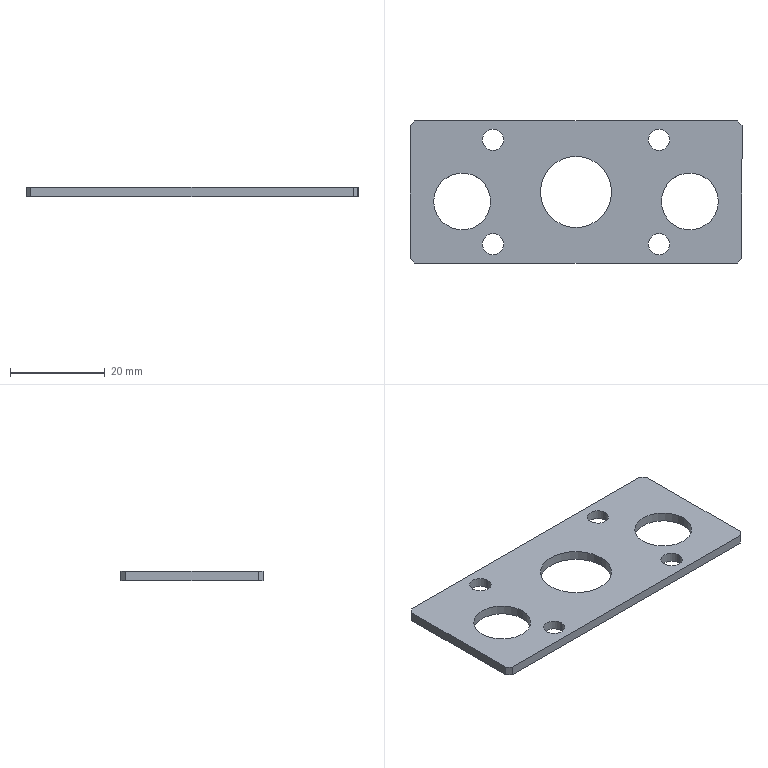Part | SolidWorks | features Chamfer 1, Extrusion 1, HoleWzd 1 | 1 solid | 24 faces | box 70 x 30 x 2 mm | volume 3263 mm3 | cylinder 14 | plane 10 | commonest cylinder face diameters 4.5 x8 12 x4 15 x2
STEP:
#1=CARTESIAN_POINT('',(-19.75,26.,0.));
#2=VERTEX_POINT('',#1);
#3=CARTESIAN_POINT('',(-15.25,26.,0.));
#4=VERTEX_POINT('',#3);
#5=CARTESIAN_POINT('',(-17.5,26.,0.));
#6=DIRECTION('',(0.,0.,1.));
#7=DIRECTION('',(1.,0.,0.));
#8=AXIS2_PLACEMENT_3D('',#5,#6,#7);
#9=CIRCLE('',#8,2.25);
#10=EDGE_CURVE('',#2,#4,#9,.T.);
#11=ORIENTED_EDGE('',*,*,#10,.F.);
#12=CARTESIAN_POINT('',(-19.75,26.,2.));
#13=VERTEX_POINT('',#12);
#14=CARTESIAN_POINT('',(-19.75,26.,2.));
#15=DIRECTION('',(0.,0.,1.));
#16=VECTOR('',#15,1000.);
#17=LINE('',#14,#16);
#18=EDGE_CURVE('',#2,#13,#17,.T.);
#19=ORIENTED_EDGE('',*,*,#18,.T.);
#20=CARTESIAN_POINT('',(-15.25,26.,2.));
#21=VERTEX_POINT('',#20);
#22=CARTESIAN_POINT('',(-17.5,26.,2.));
#23=DIRECTION('',(0.,0.,1.));
#24=DIRECTION('',(1.,0.,0.));
#25=AXIS2_PLACEMENT_3D('',#22,#23,#24);
#26=CIRCLE('',#25,2.25);
#27=EDGE_CURVE('',#13,#21,#26,.T.);
#28=ORIENTED_EDGE('',*,*,#27,.T.);
#29=CARTESIAN_POINT('',(-15.25,26.,2.));
#30=DIRECTION('',(0.,0.,1.));
#31=VECTOR('',#30,1000.);
#32=LINE('',#29,#31);
#33=EDGE_CURVE('',#4,#21,#32,.T.);
#34=ORIENTED_EDGE('',*,*,#33,.F.);
#35=EDGE_LOOP('',(#11,#19,#28,#34));
#36=FACE_OUTER_BOUND('',#35,.T.);
#37=CARTESIAN_POINT('',(-17.5,26.,2.));
#38=DIRECTION('',(0.,0.,1.));
#39=DIRECTION('',(1.,0.,0.));
#40=AXIS2_PLACEMENT_3D('',#37,#38,#39);
#41=CYLINDRICAL_SURFACE('',#40,2.25);
#42=ADVANCED_FACE('',(#36),#41,.F.);
#43=CARTESIAN_POINT('',(15.25,26.,0.));
#44=VERTEX_POINT('',#43);
#45=CARTESIAN_POINT('',(19.75,26.,0.));
#46=VERTEX_POINT('',#45);
#47=CARTESIAN_POINT('',(17.5,26.,0.));
#48=DIRECTION('',(0.,0.,1.));
#49=DIRECTION('',(1.,0.,0.));
#50=AXIS2_PLACEMENT_3D('',#47,#48,#49);
#51=CIRCLE('',#50,2.25);
#52=EDGE_CURVE('',#44,#46,#51,.T.);
#53=ORIENTED_EDGE('',*,*,#52,.F.);
#54=CARTESIAN_POINT('',(15.25,26.,2.));
#55=VERTEX_POINT('',#54);
#56=CARTESIAN_POINT('',(15.25,26.,2.));
#57=DIRECTION('',(0.,0.,1.));
#58=VECTOR('',#57,1000.);
#59=LINE('',#56,#58);
#60=EDGE_CURVE('',#44,#55,#59,.T.);
#61=ORIENTED_EDGE('',*,*,#60,.T.);
#62=CARTESIAN_POINT('',(19.75,26.,2.));
#63=VERTEX_POINT('',#62);
#64=CARTESIAN_POINT('',(17.5,26.,2.));
#65=DIRECTION('',(0.,0.,1.));
#66=DIRECTION('',(1.,0.,0.));
#67=AXIS2_PLACEMENT_3D('',#64,#65,#66);
#68=CIRCLE('',#67,2.25);
#69=EDGE_CURVE('',#55,#63,#68,.T.);
#70=ORIENTED_EDGE('',*,*,#69,.T.);
#71=CARTESIAN_POINT('',(19.75,26.,2.));
#72=DIRECTION('',(0.,0.,1.));
#73=VECTOR('',#72,1000.);
#74=LINE('',#71,#73);
#75=EDGE_CURVE('',#46,#63,#74,.T.);
#76=ORIENTED_EDGE('',*,*,#75,.F.);
#77=EDGE_LOOP('',(#53,#61,#70,#76));
#78=FACE_OUTER_BOUND('',#77,.T.);
#79=CARTESIAN_POINT('',(17.5,26.,2.));
#80=DIRECTION('',(0.,0.,1.));
#81=DIRECTION('',(1.,0.,0.));
#82=AXIS2_PLACEMENT_3D('',#79,#80,#81);
#83=CYLINDRICAL_SURFACE('',#82,2.25);
#84=ADVANCED_FACE('',(#78),#83,.F.);
#85=CARTESIAN_POINT('',(-19.75,4.,0.));
#86=VERTEX_POINT('',#85);
#87=CARTESIAN_POINT('',(-15.25,4.,0.));
#88=VERTEX_POINT('',#87);
#89=CARTESIAN_POINT('',(-17.5,4.,0.));
#90=DIRECTION('',(0.,0.,1.));
#91=DIRECTION('',(1.,0.,0.));
#92=AXIS2_PLACEMENT_3D('',#89,#90,#91);
#93=CIRCLE('',#92,2.25);
#94=EDGE_CURVE('',#86,#88,#93,.T.);
#95=ORIENTED_EDGE('',*,*,#94,.F.);
#96=CARTESIAN_POINT('',(-19.75,4.,2.));
#97=VERTEX_POINT('',#96);
#98=CARTESIAN_POINT('',(-19.75,4.,2.));
#99=DIRECTION('',(0.,0.,1.));
#100=VECTOR('',#99,1000.);
#101=LINE('',#98,#100);
#102=EDGE_CURVE('',#86,#97,#101,.T.);
#103=ORIENTED_EDGE('',*,*,#102,.T.);
#104=CARTESIAN_POINT('',(-15.25,4.,2.));
#105=VERTEX_POINT('',#104);
#106=CARTESIAN_POINT('',(-17.5,4.,2.));
#107=DIRECTION('',(0.,0.,1.));
#108=DIRECTION('',(1.,0.,0.));
#109=AXIS2_PLACEMENT_3D('',#106,#107,#108);
#110=CIRCLE('',#109,2.25);
#111=EDGE_CURVE('',#97,#105,#110,.T.);
#112=ORIENTED_EDGE('',*,*,#111,.T.);
#113=CARTESIAN_POINT('',(-15.25,4.,2.));
#114=DIRECTION('',(0.,0.,1.));
#115=VECTOR('',#114,1000.);
#116=LINE('',#113,#115);
#117=EDGE_CURVE('',#88,#105,#116,.T.);
#118=ORIENTED_EDGE('',*,*,#117,.F.);
#119=EDGE_LOOP('',(#95,#103,#112,#118));
#120=FACE_OUTER_BOUND('',#119,.T.);
#121=CARTESIAN_POINT('',(-17.5,4.,2.));
#122=DIRECTION('',(0.,0.,1.));
#123=DIRECTION('',(1.,0.,0.));
#124=AXIS2_PLACEMENT_3D('',#121,#122,#123);
#125=CYLINDRICAL_SURFACE('',#124,2.25);
#126=ADVANCED_FACE('',(#120),#125,.F.);
#127=CARTESIAN_POINT('',(15.25,4.,0.));
#128=VERTEX_POINT('',#127);
#129=CARTESIAN_POINT('',(19.75,4.,0.));
#130=VERTEX_POINT('',#129);
#131=CARTESIAN_POINT('',(17.5,4.,0.));
#132=DIRECTION('',(0.,0.,1.));
#133=DIRECTION('',(1.,0.,0.));
#134=AXIS2_PLACEMENT_3D('',#131,#132,#133);
#135=CIRCLE('',#134,2.25);
#136=EDGE_CURVE('',#128,#130,#135,.T.);
#137=ORIENTED_EDGE('',*,*,#136,.F.);
#138=CARTESIAN_POINT('',(15.25,4.,2.));
#139=VERTEX_POINT('',#138);
#140=CARTESIAN_POINT('',(15.25,4.,2.));
#141=DIRECTION('',(0.,0.,1.));
#142=VECTOR('',#141,1000.);
#143=LINE('',#140,#142);
#144=EDGE_CURVE('',#128,#139,#143,.T.);
#145=ORIENTED_EDGE('',*,*,#144,.T.);
#146=CARTESIAN_POINT('',(19.75,4.,2.));
#147=VERTEX_POINT('',#146);
#148=CARTESIAN_POINT('',(17.5,4.,2.));
#149=DIRECTION('',(0.,0.,1.));
#150=DIRECTION('',(1.,0.,0.));
#151=AXIS2_PLACEMENT_3D('',#148,#149,#150);
#152=CIRCLE('',#151,2.25);
#153=EDGE_CURVE('',#139,#147,#152,.T.);
#154=ORIENTED_EDGE('',*,*,#153,.T.);
#155=CARTESIAN_POINT('',(19.75,4.,2.));
#156=DIRECTION('',(0.,0.,1.));
#157=VECTOR('',#156,1000.);
#158=LINE('',#155,#157);
#159=EDGE_CURVE('',#130,#147,#158,.T.);
#160=ORIENTED_EDGE('',*,*,#159,.F.);
#161=EDGE_LOOP('',(#137,#145,#154,#160));
#162=FACE_OUTER_BOUND('',#161,.T.);
#163=CARTESIAN_POINT('',(17.5,4.,2.));
#164=DIRECTION('',(0.,0.,1.));
#165=DIRECTION('',(1.,0.,0.));
#166=AXIS2_PLACEMENT_3D('',#163,#164,#165);
#167=CYLINDRICAL_SURFACE('',#166,2.25);
#168=ADVANCED_FACE('',(#162),#167,.F.);
#169=CARTESIAN_POINT('',(-7.5,15.,2.));
#170=VERTEX_POINT('',#169);
#171=CARTESIAN_POINT('',(7.5,15.,2.));
#172=VERTEX_POINT('',#171);
#173=CARTESIAN_POINT('',(0.,15.,2.));
#174=DIRECTION('',(0.,0.,1.));
#175=DIRECTION('',(1.,0.,0.));
#176=AXIS2_PLACEMENT_3D('',#173,#174,#175);
#177=CIRCLE('',#176,7.5);
#178=EDGE_CURVE('',#170,#172,#177,.T.);
#179=ORIENTED_EDGE('',*,*,#178,.T.);
#180=CARTESIAN_POINT('',(7.5,15.,0.));
#181=VERTEX_POINT('',#180);
#182=CARTESIAN_POINT('',(7.5,15.,2.));
#183=DIRECTION('',(0.,0.,-1.));
#184=VECTOR('',#183,1000.);
#185=LINE('',#182,#184);
#186=EDGE_CURVE('',#172,#181,#185,.T.);
#187=ORIENTED_EDGE('',*,*,#186,.T.);
#188=CARTESIAN_POINT('',(-7.5,15.,0.));
#189=VERTEX_POINT('',#188);
#190=CARTESIAN_POINT('',(0.,15.,0.));
#191=DIRECTION('',(0.,0.,1.));
#192=DIRECTION('',(1.,0.,0.));
#193=AXIS2_PLACEMENT_3D('',#190,#191,#192);
#194=CIRCLE('',#193,7.5);
#195=EDGE_CURVE('',#189,#181,#194,.T.);
#196=ORIENTED_EDGE('',*,*,#195,.F.);
#197=CARTESIAN_POINT('',(-7.5,15.,2.));
#198=DIRECTION('',(0.,0.,-1.));
#199=VECTOR('',#198,1000.);
#200=LINE('',#197,#199);
#201=EDGE_CURVE('',#170,#189,#200,.T.);
#202=ORIENTED_EDGE('',*,*,#201,.F.);
#203=EDGE_LOOP('',(#179,#187,#196,#202));
#204=FACE_OUTER_BOUND('',#203,.T.);
#205=CARTESIAN_POINT('',(0.,15.,2.));
#206=DIRECTION('',(0.,0.,-1.));
#207=DIRECTION('',(-1.,0.,0.));
#208=AXIS2_PLACEMENT_3D('',#205,#206,#207);
#209=CYLINDRICAL_SURFACE('',#208,7.5);
#210=ADVANCED_FACE('',(#204),#209,.F.);
#211=CARTESIAN_POINT('',(18.,13.,2.));
#212=VERTEX_POINT('',#211);
#213=CARTESIAN_POINT('',(30.,13.,2.));
#214=VERTEX_POINT('',#213);
#215=CARTESIAN_POINT('',(24.,13.,2.));
#216=DIRECTION('',(0.,0.,1.));
#217=DIRECTION('',(1.,0.,0.));
#218=AXIS2_PLACEMENT_3D('',#215,#216,#217);
#219=CIRCLE('',#218,6.);
#220=EDGE_CURVE('',#212,#214,#219,.T.);
#221=ORIENTED_EDGE('',*,*,#220,.T.);
#222=CARTESIAN_POINT('',(30.,13.,0.));
#223=VERTEX_POINT('',#222);
#224=CARTESIAN_POINT('',(30.,13.,2.));
#225=DIRECTION('',(0.,0.,-1.));
#226=VECTOR('',#225,1000.);
#227=LINE('',#224,#226);
#228=EDGE_CURVE('',#214,#223,#227,.T.);
#229=ORIENTED_EDGE('',*,*,#228,.T.);
#230=CARTESIAN_POINT('',(18.,13.,0.));
#231=VERTEX_POINT('',#230);
#232=CARTESIAN_POINT('',(24.,13.,0.));
#233=DIRECTION('',(0.,0.,1.));
#234=DIRECTION('',(1.,0.,0.));
#235=AXIS2_PLACEMENT_3D('',#232,#233,#234);
#236=CIRCLE('',#235,6.);
#237=EDGE_CURVE('',#231,#223,#236,.T.);
#238=ORIENTED_EDGE('',*,*,#237,.F.);
#239=CARTESIAN_POINT('',(18.,13.,2.));
#240=DIRECTION('',(0.,0.,-1.));
#241=VECTOR('',#240,1000.);
#242=LINE('',#239,#241);
#243=EDGE_CURVE('',#212,#231,#242,.T.);
#244=ORIENTED_EDGE('',*,*,#243,.F.);
#245=EDGE_LOOP('',(#221,#229,#238,#244));
#246=FACE_OUTER_BOUND('',#245,.T.);
#247=CARTESIAN_POINT('',(24.,13.,2.));
#248=DIRECTION('',(0.,0.,-1.));
#249=DIRECTION('',(-1.,0.,0.));
#250=AXIS2_PLACEMENT_3D('',#247,#248,#249);
#251=CYLINDRICAL_SURFACE('',#250,6.);
#252=ADVANCED_FACE('',(#246),#251,.F.);
#253=CARTESIAN_POINT('',(-30.,13.,2.));
#254=VERTEX_POINT('',#253);
#255=CARTESIAN_POINT('',(-18.,13.,2.));
#256=VERTEX_POINT('',#255);
#257=CARTESIAN_POINT('',(-24.,13.,2.));
#258=DIRECTION('',(0.,0.,1.));
#259=DIRECTION('',(1.,0.,0.));
#260=AXIS2_PLACEMENT_3D('',#257,#258,#259);
#261=CIRCLE('',#260,6.);
#262=EDGE_CURVE('',#254,#256,#261,.T.);
#263=ORIENTED_EDGE('',*,*,#262,.T.);
#264=CARTESIAN_POINT('',(-18.,13.,0.));
#265=VERTEX_POINT('',#264);
#266=CARTESIAN_POINT('',(-18.,13.,2.));
#267=DIRECTION('',(0.,0.,-1.));
#268=VECTOR('',#267,1000.);
#269=LINE('',#266,#268);
#270=EDGE_CURVE('',#256,#265,#269,.T.);
#271=ORIENTED_EDGE('',*,*,#270,.T.);
#272=CARTESIAN_POINT('',(-30.,13.,0.));
#273=VERTEX_POINT('',#272);
#274=CARTESIAN_POINT('',(-24.,13.,0.));
#275=DIRECTION('',(0.,0.,1.));
#276=DIRECTION('',(1.,0.,0.));
#277=AXIS2_PLACEMENT_3D('',#274,#275,#276);
#278=CIRCLE('',#277,6.);
#279=EDGE_CURVE('',#273,#265,#278,.T.);
#280=ORIENTED_EDGE('',*,*,#279,.F.);
#281=CARTESIAN_POINT('',(-30.,13.,2.));
#282=DIRECTION('',(0.,0.,-1.));
#283=VECTOR('',#282,1000.);
#284=LINE('',#281,#283);
#285=EDGE_CURVE('',#254,#273,#284,.T.);
#286=ORIENTED_EDGE('',*,*,#285,.F.);
#287=EDGE_LOOP('',(#263,#271,#280,#286));
#288=FACE_OUTER_BOUND('',#287,.T.);
#289=CARTESIAN_POINT('',(-24.,13.,2.));
#290=DIRECTION('',(0.,0.,-1.));
#291=DIRECTION('',(-1.,0.,0.));
#292=AXIS2_PLACEMENT_3D('',#289,#290,#291);
#293=CYLINDRICAL_SURFACE('',#292,6.);
#294=ADVANCED_FACE('',(#288),#293,.F.);
#295=CARTESIAN_POINT('',(-17.5,26.,2.));
#296=DIRECTION('',(0.,0.,1.));
#297=DIRECTION('',(1.,0.,0.));
#298=AXIS2_PLACEMENT_3D('',#295,#296,#297);
#299=CIRCLE('',#298,2.25);
#300=EDGE_CURVE('',#21,#13,#299,.T.);
#301=ORIENTED_EDGE('',*,*,#300,.F.);
#302=ORIENTED_EDGE('',*,*,#27,.F.);
#303=EDGE_LOOP('',(#301,#302));
#304=FACE_BOUND('',#303,.T.);
#305=CARTESIAN_POINT('',(17.5,26.,2.));
#306=DIRECTION('',(0.,0.,1.));
#307=DIRECTION('',(1.,0.,0.));
#308=AXIS2_PLACEMENT_3D('',#305,#306,#307);
#309=CIRCLE('',#308,2.25);
#310=EDGE_CURVE('',#63,#55,#309,.T.);
#311=ORIENTED_EDGE('',*,*,#310,.F.);
#312=ORIENTED_EDGE('',*,*,#69,.F.);
#313=EDGE_LOOP('',(#311,#312));
#314=FACE_BOUND('',#313,.T.);
#315=CARTESIAN_POINT('',(-17.5,4.,2.));
#316=DIRECTION('',(0.,0.,1.));
#317=DIRECTION('',(1.,0.,0.));
#318=AXIS2_PLACEMENT_3D('',#315,#316,#317);
#319=CIRCLE('',#318,2.25);
#320=EDGE_CURVE('',#105,#97,#319,.T.);
#321=ORIENTED_EDGE('',*,*,#320,.F.);
#322=ORIENTED_EDGE('',*,*,#111,.F.);
#323=EDGE_LOOP('',(#321,#322));
#324=FACE_BOUND('',#323,.T.);
#325=CARTESIAN_POINT('',(17.5,4.,2.));
#326=DIRECTION('',(0.,0.,1.));
#327=DIRECTION('',(1.,0.,0.));
#328=AXIS2_PLACEMENT_3D('',#325,#326,#327);
#329=CIRCLE('',#328,2.25);
#330=EDGE_CURVE('',#147,#139,#329,.T.);
#331=ORIENTED_EDGE('',*,*,#330,.F.);
#332=ORIENTED_EDGE('',*,*,#153,.F.);
#333=EDGE_LOOP('',(#331,#332));
#334=FACE_BOUND('',#333,.T.);
#335=ORIENTED_EDGE('',*,*,#220,.F.);
#336=CARTESIAN_POINT('',(24.,13.,2.));
#337=DIRECTION('',(0.,0.,1.));
#338=DIRECTION('',(1.,0.,0.));
#339=AXIS2_PLACEMENT_3D('',#336,#337,#338);
#340=CIRCLE('',#339,6.);
#341=EDGE_CURVE('',#214,#212,#340,.T.);
#342=ORIENTED_EDGE('',*,*,#341,.F.);
#343=EDGE_LOOP('',(#335,#342));
#344=FACE_BOUND('',#343,.T.);
#345=CARTESIAN_POINT('',(-35.,29.,2.));
#346=VERTEX_POINT('',#345);
#347=CARTESIAN_POINT('',(-35.,1.,2.));
#348=VERTEX_POINT('',#347);
#349=CARTESIAN_POINT('',(-35.,30.,2.));
#350=DIRECTION('',(0.,-1.,0.));
#351=VECTOR('',#350,1000.);
#352=LINE('',#349,#351);
#353=EDGE_CURVE('',#346,#348,#352,.T.);
#354=ORIENTED_EDGE('',*,*,#353,.T.);
#355=CARTESIAN_POINT('',(-34.,0.,2.));
#356=VERTEX_POINT('',#355);
#357=CARTESIAN_POINT('',(-34.,0.,2.));
#358=DIRECTION('',(0.7071,-0.7071,0.));
#359=VECTOR('',#358,1000.);
#360=LINE('',#357,#359);
#361=EDGE_CURVE('',#348,#356,#360,.T.);
#362=ORIENTED_EDGE('',*,*,#361,.T.);
#363=CARTESIAN_POINT('',(34.,0.,2.));
#364=VERTEX_POINT('',#363);
#365=CARTESIAN_POINT('',(35.,0.,2.));
#366=DIRECTION('',(1.,0.,0.));
#367=VECTOR('',#366,1000.);
#368=LINE('',#365,#367);
#369=EDGE_CURVE('',#356,#364,#368,.T.);
#370=ORIENTED_EDGE('',*,*,#369,.T.);
#371=CARTESIAN_POINT('',(35.,1.,2.));
#372=VERTEX_POINT('',#371);
#373=CARTESIAN_POINT('',(35.,1.,2.));
#374=DIRECTION('',(0.7071,0.7071,0.));
#375=VECTOR('',#374,1000.);
#376=LINE('',#373,#375);
#377=EDGE_CURVE('',#364,#372,#376,.T.);
#378=ORIENTED_EDGE('',*,*,#377,.T.);
#379=CARTESIAN_POINT('',(35.,29.,2.));
#380=VERTEX_POINT('',#379);
#381=CARTESIAN_POINT('',(35.,30.,2.));
#382=DIRECTION('',(0.,1.,0.));
#383=VECTOR('',#382,1000.);
#384=LINE('',#381,#383);
#385=EDGE_CURVE('',#372,#380,#384,.T.);
#386=ORIENTED_EDGE('',*,*,#385,.T.);
#387=CARTESIAN_POINT('',(34.,30.,2.));
#388=VERTEX_POINT('',#387);
#389=CARTESIAN_POINT('',(34.,30.,2.));
#390=DIRECTION('',(-0.7071,0.7071,0.));
#391=VECTOR('',#390,1000.);
#392=LINE('',#389,#391);
#393=EDGE_CURVE('',#380,#388,#392,.T.);
#394=ORIENTED_EDGE('',*,*,#393,.T.);
#395=CARTESIAN_POINT('',(-34.,30.,2.));
#396=VERTEX_POINT('',#395);
#397=CARTESIAN_POINT('',(35.,30.,2.));
#398=DIRECTION('',(-1.,0.,0.));
#399=VECTOR('',#398,1000.);
#400=LINE('',#397,#399);
#401=EDGE_CURVE('',#388,#396,#400,.T.);
#402=ORIENTED_EDGE('',*,*,#401,.T.);
#403=CARTESIAN_POINT('',(-35.,29.,2.));
#404=DIRECTION('',(-0.7071,-0.7071,0.));
#405=VECTOR('',#404,1000.);
#406=LINE('',#403,#405);
#407=EDGE_CURVE('',#396,#346,#406,.T.);
#408=ORIENTED_EDGE('',*,*,#407,.T.);
#409=EDGE_LOOP('',(#354,#362,#370,#378,#386,#394,#402,#408));
#410=FACE_OUTER_BOUND('',#409,.T.);
#411=ORIENTED_EDGE('',*,*,#262,.F.);
#412=CARTESIAN_POINT('',(-24.,13.,2.));
#413=DIRECTION('',(0.,0.,1.));
#414=DIRECTION('',(1.,0.,0.));
#415=AXIS2_PLACEMENT_3D('',#412,#413,#414);
#416=CIRCLE('',#415,6.);
#417=EDGE_CURVE('',#256,#254,#416,.T.);
#418=ORIENTED_EDGE('',*,*,#417,.F.);
#419=EDGE_LOOP('',(#411,#418));
#420=FACE_BOUND('',#419,.T.);
#421=ORIENTED_EDGE('',*,*,#178,.F.);
#422=CARTESIAN_POINT('',(0.,15.,2.));
#423=DIRECTION('',(0.,0.,1.));
#424=DIRECTION('',(1.,0.,0.));
#425=AXIS2_PLACEMENT_3D('',#422,#423,#424);
#426=CIRCLE('',#425,7.5);
#427=EDGE_CURVE('',#172,#170,#426,.T.);
#428=ORIENTED_EDGE('',*,*,#427,.F.);
#429=EDGE_LOOP('',(#421,#428));
#430=FACE_BOUND('',#429,.T.);
#431=CARTESIAN_POINT('',(35.,0.,2.));
#432=DIRECTION('',(0.,0.,-1.));
#433=DIRECTION('',(-1.,0.,0.));
#434=AXIS2_PLACEMENT_3D('',#431,#432,#433);
#435=PLANE('',#434);
#436=ADVANCED_FACE('',(#304,#314,#324,#334,#344,#410,#420,#430),#435,.F.);
#437=CARTESIAN_POINT('',(-17.5,26.,0.));
#438=DIRECTION('',(0.,0.,1.));
#439=DIRECTION('',(1.,0.,0.));
#440=AXIS2_PLACEMENT_3D('',#437,#438,#439);
#441=CIRCLE('',#440,2.25);
#442=EDGE_CURVE('',#4,#2,#441,.T.);
#443=ORIENTED_EDGE('',*,*,#442,.T.);
#444=ORIENTED_EDGE('',*,*,#10,.T.);
#445=EDGE_LOOP('',(#443,#444));
#446=FACE_BOUND('',#445,.T.);
#447=CARTESIAN_POINT('',(17.5,26.,0.));
#448=DIRECTION('',(0.,0.,1.));
#449=DIRECTION('',(1.,0.,0.));
#450=AXIS2_PLACEMENT_3D('',#447,#448,#449);
#451=CIRCLE('',#450,2.25);
#452=EDGE_CURVE('',#46,#44,#451,.T.);
#453=ORIENTED_EDGE('',*,*,#452,.T.);
#454=ORIENTED_EDGE('',*,*,#52,.T.);
#455=EDGE_LOOP('',(#453,#454));
#456=FACE_BOUND('',#455,.T.);
#457=CARTESIAN_POINT('',(-17.5,4.,0.));
#458=DIRECTION('',(0.,0.,1.));
#459=DIRECTION('',(1.,0.,0.));
#460=AXIS2_PLACEMENT_3D('',#457,#458,#459);
#461=CIRCLE('',#460,2.25);
#462=EDGE_CURVE('',#88,#86,#461,.T.);
#463=ORIENTED_EDGE('',*,*,#462,.T.);
#464=ORIENTED_EDGE('',*,*,#94,.T.);
#465=EDGE_LOOP('',(#463,#464));
#466=FACE_BOUND('',#465,.T.);
#467=CARTESIAN_POINT('',(17.5,4.,0.));
#468=DIRECTION('',(0.,0.,1.));
#469=DIRECTION('',(1.,0.,0.));
#470=AXIS2_PLACEMENT_3D('',#467,#468,#469);
#471=CIRCLE('',#470,2.25);
#472=EDGE_CURVE('',#130,#128,#471,.T.);
#473=ORIENTED_EDGE('',*,*,#472,.T.);
#474=ORIENTED_EDGE('',*,*,#136,.T.);
#475=EDGE_LOOP('',(#473,#474));
#476=FACE_BOUND('',#475,.T.);
#477=ORIENTED_EDGE('',*,*,#237,.T.);
#478=CARTESIAN_POINT('',(24.,13.,0.));
#479=DIRECTION('',(0.,0.,1.));
#480=DIRECTION('',(1.,0.,0.));
#481=AXIS2_PLACEMENT_3D('',#478,#479,#480);
#482=CIRCLE('',#481,6.);
#483=EDGE_CURVE('',#223,#231,#482,.T.);
#484=ORIENTED_EDGE('',*,*,#483,.T.);
#485=EDGE_LOOP('',(#477,#484));
#486=FACE_BOUND('',#485,.T.);
#487=CARTESIAN_POINT('',(-34.,0.,0.));
#488=VERTEX_POINT('',#487);
#489=CARTESIAN_POINT('',(34.,0.,0.));
#490=VERTEX_POINT('',#489);
#491=CARTESIAN_POINT('',(35.,0.,0.));
#492=DIRECTION('',(1.,0.,0.));
#493=VECTOR('',#492,1000.);
#494=LINE('',#491,#493);
#495=EDGE_CURVE('',#488,#490,#494,.T.);
#496=ORIENTED_EDGE('',*,*,#495,.F.);
#497=CARTESIAN_POINT('',(-35.,1.,0.));
#498=VERTEX_POINT('',#497);
#499=CARTESIAN_POINT('',(0.5,-34.5,0.));
#500=DIRECTION('',(-0.7071,0.7071,0.));
#501=VECTOR('',#500,1000.);
#502=LINE('',#499,#501);
#503=EDGE_CURVE('',#488,#498,#502,.T.);
#504=ORIENTED_EDGE('',*,*,#503,.T.);
#505=CARTESIAN_POINT('',(-35.,29.,0.));
#506=VERTEX_POINT('',#505);
#507=CARTESIAN_POINT('',(-35.,30.,0.));
#508=DIRECTION('',(0.,-1.,0.));
#509=VECTOR('',#508,1000.);
#510=LINE('',#507,#509);
#511=EDGE_CURVE('',#506,#498,#510,.T.);
#512=ORIENTED_EDGE('',*,*,#511,.F.);
#513=CARTESIAN_POINT('',(-34.,30.,0.));
#514=VERTEX_POINT('',#513);
#515=CARTESIAN_POINT('',(-14.5,49.5,0.));
#516=DIRECTION('',(0.7071,0.7071,0.));
#517=VECTOR('',#516,1000.);
#518=LINE('',#515,#517);
#519=EDGE_CURVE('',#506,#514,#518,.T.);
#520=ORIENTED_EDGE('',*,*,#519,.T.);
#521=CARTESIAN_POINT('',(34.,30.,0.));
#522=VERTEX_POINT('',#521);
#523=CARTESIAN_POINT('',(35.,30.,0.));
#524=DIRECTION('',(-1.,0.,0.));
#525=VECTOR('',#524,1000.);
#526=LINE('',#523,#525);
#527=EDGE_CURVE('',#522,#514,#526,.T.);
#528=ORIENTED_EDGE('',*,*,#527,.F.);
#529=CARTESIAN_POINT('',(35.,29.,0.));
#530=VERTEX_POINT('',#529);
#531=CARTESIAN_POINT('',(49.5,14.5,0.));
#532=DIRECTION('',(0.7071,-0.7071,0.));
#533=VECTOR('',#532,1000.);
#534=LINE('',#531,#533);
#535=EDGE_CURVE('',#522,#530,#534,.T.);
#536=ORIENTED_EDGE('',*,*,#535,.T.);
#537=CARTESIAN_POINT('',(35.,1.,0.));
#538=VERTEX_POINT('',#537);
#539=CARTESIAN_POINT('',(35.,30.,0.));
#540=DIRECTION('',(0.,1.,0.));
#541=VECTOR('',#540,1000.);
#542=LINE('',#539,#541);
#543=EDGE_CURVE('',#538,#530,#542,.T.);
#544=ORIENTED_EDGE('',*,*,#543,.F.);
#545=CARTESIAN_POINT('',(34.5,0.5,0.));
#546=DIRECTION('',(-0.7071,-0.7071,0.));
#547=VECTOR('',#546,1000.);
#548=LINE('',#545,#547);
#549=EDGE_CURVE('',#538,#490,#548,.T.);
#550=ORIENTED_EDGE('',*,*,#549,.T.);
#551=EDGE_LOOP('',(#496,#504,#512,#520,#528,#536,#544,#550));
#552=FACE_OUTER_BOUND('',#551,.T.);
#553=ORIENTED_EDGE('',*,*,#279,.T.);
#554=CARTESIAN_POINT('',(-24.,13.,0.));
#555=DIRECTION('',(0.,0.,1.));
#556=DIRECTION('',(1.,0.,0.));
#557=AXIS2_PLACEMENT_3D('',#554,#555,#556);
#558=CIRCLE('',#557,6.);
#559=EDGE_CURVE('',#265,#273,#558,.T.);
#560=ORIENTED_EDGE('',*,*,#559,.T.);
#561=EDGE_LOOP('',(#553,#560));
#562=FACE_BOUND('',#561,.T.);
#563=ORIENTED_EDGE('',*,*,#195,.T.);
#564=CARTESIAN_POINT('',(0.,15.,0.));
#565=DIRECTION('',(0.,0.,1.));
#566=DIRECTION('',(1.,0.,0.));
#567=AXIS2_PLACEMENT_3D('',#564,#565,#566);
#568=CIRCLE('',#567,7.5);
#569=EDGE_CURVE('',#181,#189,#568,.T.);
#570=ORIENTED_EDGE('',*,*,#569,.T.);
#571=EDGE_LOOP('',(#563,#570));
#572=FACE_BOUND('',#571,.T.);
#573=CARTESIAN_POINT('',(35.,0.,0.));
#574=DIRECTION('',(0.,0.,-1.));
#575=DIRECTION('',(-1.,0.,0.));
#576=AXIS2_PLACEMENT_3D('',#573,#574,#575);
#577=PLANE('',#576);
#578=ADVANCED_FACE('',(#446,#456,#466,#476,#486,#552,#562,#572),#577,.T.);
#579=ORIENTED_EDGE('',*,*,#543,.T.);
#580=CARTESIAN_POINT('',(35.,29.,2.));
#581=DIRECTION('',(0.,0.,1.));
#582=VECTOR('',#581,1000.);
#583=LINE('',#580,#582);
#584=EDGE_CURVE('',#530,#380,#583,.T.);
#585=ORIENTED_EDGE('',*,*,#584,.T.);
#586=ORIENTED_EDGE('',*,*,#385,.F.);
#587=CARTESIAN_POINT('',(35.,1.,2.));
#588=DIRECTION('',(0.,0.,-1.));
#589=VECTOR('',#588,1000.);
#590=LINE('',#587,#589);
#591=EDGE_CURVE('',#372,#538,#590,.T.);
#592=ORIENTED_EDGE('',*,*,#591,.T.);
#593=EDGE_LOOP('',(#579,#585,#586,#592));
#594=FACE_OUTER_BOUND('',#593,.T.);
#595=CARTESIAN_POINT('',(35.,30.,2.));
#596=DIRECTION('',(-1.,0.,0.));
#597=DIRECTION('',(0.,-1.,0.));
#598=AXIS2_PLACEMENT_3D('',#595,#596,#597);
#599=PLANE('',#598);
#600=ADVANCED_FACE('',(#594),#599,.F.);
#601=ORIENTED_EDGE('',*,*,#527,.T.);
#602=CARTESIAN_POINT('',(-34.,30.,2.));
#603=DIRECTION('',(0.,0.,1.));
#604=VECTOR('',#603,1000.);
#605=LINE('',#602,#604);
#606=EDGE_CURVE('',#514,#396,#605,.T.);
#607=ORIENTED_EDGE('',*,*,#606,.T.);
#608=ORIENTED_EDGE('',*,*,#401,.F.);
#609=CARTESIAN_POINT('',(34.,30.,2.));
#610=DIRECTION('',(0.,0.,-1.));
#611=VECTOR('',#610,1000.);
#612=LINE('',#609,#611);
#613=EDGE_CURVE('',#388,#522,#612,.T.);
#614=ORIENTED_EDGE('',*,*,#613,.T.);
#615=EDGE_LOOP('',(#601,#607,#608,#614));
#616=FACE_OUTER_BOUND('',#615,.T.);
#617=CARTESIAN_POINT('',(35.,30.,2.));
#618=DIRECTION('',(0.,-1.,0.));
#619=DIRECTION('',(0.,0.,-1.));
#620=AXIS2_PLACEMENT_3D('',#617,#618,#619);
#621=PLANE('',#620);
#622=ADVANCED_FACE('',(#616),#621,.F.);
#623=ORIENTED_EDGE('',*,*,#511,.T.);
#624=CARTESIAN_POINT('',(-35.,1.,2.));
#625=DIRECTION('',(0.,0.,1.));
#626=VECTOR('',#625,1000.);
#627=LINE('',#624,#626);
#628=EDGE_CURVE('',#498,#348,#627,.T.);
#629=ORIENTED_EDGE('',*,*,#628,.T.);
#630=ORIENTED_EDGE('',*,*,#353,.F.);
#631=CARTESIAN_POINT('',(-35.,29.,2.));
#632=DIRECTION('',(0.,0.,-1.));
#633=VECTOR('',#632,1000.);
#634=LINE('',#631,#633);
#635=EDGE_CURVE('',#346,#506,#634,.T.);
#636=ORIENTED_EDGE('',*,*,#635,.T.);
#637=EDGE_LOOP('',(#623,#629,#630,#636));
#638=FACE_OUTER_BOUND('',#637,.T.);
#639=CARTESIAN_POINT('',(-35.,30.,2.));
#640=DIRECTION('',(1.,0.,0.));
#641=DIRECTION('',(0.,1.,0.));
#642=AXIS2_PLACEMENT_3D('',#639,#640,#641);
#643=PLANE('',#642);
#644=ADVANCED_FACE('',(#638),#643,.F.);
#645=ORIENTED_EDGE('',*,*,#369,.F.);
#646=CARTESIAN_POINT('',(-34.,0.,2.));
#647=DIRECTION('',(0.,0.,-1.));
#648=VECTOR('',#647,1000.);
#649=LINE('',#646,#648);
#650=EDGE_CURVE('',#356,#488,#649,.T.);
#651=ORIENTED_EDGE('',*,*,#650,.T.);
#652=ORIENTED_EDGE('',*,*,#495,.T.);
#653=CARTESIAN_POINT('',(34.,0.,2.));
#654=DIRECTION('',(0.,0.,1.));
#655=VECTOR('',#654,1000.);
#656=LINE('',#653,#655);
#657=EDGE_CURVE('',#490,#364,#656,.T.);
#658=ORIENTED_EDGE('',*,*,#657,.T.);
#659=EDGE_LOOP('',(#645,#651,#652,#658));
#660=FACE_OUTER_BOUND('',#659,.T.);
#661=CARTESIAN_POINT('',(35.,0.,2.));
#662=DIRECTION('',(0.,1.,0.));
#663=DIRECTION('',(0.,0.,1.));
#664=AXIS2_PLACEMENT_3D('',#661,#662,#663);
#665=PLANE('',#664);
#666=ADVANCED_FACE('',(#660),#665,.F.);
#667=ORIENTED_EDGE('',*,*,#270,.F.);
#668=ORIENTED_EDGE('',*,*,#417,.T.);
#669=ORIENTED_EDGE('',*,*,#285,.T.);
#670=ORIENTED_EDGE('',*,*,#559,.F.);
#671=EDGE_LOOP('',(#667,#668,#669,#670));
#672=FACE_OUTER_BOUND('',#671,.T.);
#673=CARTESIAN_POINT('',(-24.,13.,2.));
#674=DIRECTION('',(0.,0.,-1.));
#675=DIRECTION('',(-1.,0.,0.));
#676=AXIS2_PLACEMENT_3D('',#673,#674,#675);
#677=CYLINDRICAL_SURFACE('',#676,6.);
#678=ADVANCED_FACE('',(#672),#677,.F.);
#679=ORIENTED_EDGE('',*,*,#228,.F.);
#680=ORIENTED_EDGE('',*,*,#341,.T.);
#681=ORIENTED_EDGE('',*,*,#243,.T.);
#682=ORIENTED_EDGE('',*,*,#483,.F.);
#683=EDGE_LOOP('',(#679,#680,#681,#682));
#684=FACE_OUTER_BOUND('',#683,.T.);
#685=CARTESIAN_POINT('',(24.,13.,2.));
#686=DIRECTION('',(0.,0.,-1.));
#687=DIRECTION('',(-1.,0.,0.));
#688=AXIS2_PLACEMENT_3D('',#685,#686,#687);
#689=CYLINDRICAL_SURFACE('',#688,6.);
#690=ADVANCED_FACE('',(#684),#689,.F.);
#691=ORIENTED_EDGE('',*,*,#186,.F.);
#692=ORIENTED_EDGE('',*,*,#427,.T.);
#693=ORIENTED_EDGE('',*,*,#201,.T.);
#694=ORIENTED_EDGE('',*,*,#569,.F.);
#695=EDGE_LOOP('',(#691,#692,#693,#694));
#696=FACE_OUTER_BOUND('',#695,.T.);
#697=CARTESIAN_POINT('',(0.,15.,2.));
#698=DIRECTION('',(0.,0.,-1.));
#699=DIRECTION('',(-1.,0.,0.));
#700=AXIS2_PLACEMENT_3D('',#697,#698,#699);
#701=CYLINDRICAL_SURFACE('',#700,7.5);
#702=ADVANCED_FACE('',(#696),#701,.F.);
#703=ORIENTED_EDGE('',*,*,#144,.F.);
#704=ORIENTED_EDGE('',*,*,#472,.F.);
#705=ORIENTED_EDGE('',*,*,#159,.T.);
#706=ORIENTED_EDGE('',*,*,#330,.T.);
#707=EDGE_LOOP('',(#703,#704,#705,#706));
#708=FACE_OUTER_BOUND('',#707,.T.);
#709=CARTESIAN_POINT('',(17.5,4.,2.));
#710=DIRECTION('',(0.,0.,1.));
#711=DIRECTION('',(1.,0.,0.));
#712=AXIS2_PLACEMENT_3D('',#709,#710,#711);
#713=CYLINDRICAL_SURFACE('',#712,2.25);
#714=ADVANCED_FACE('',(#708),#713,.F.);
#715=ORIENTED_EDGE('',*,*,#102,.F.);
#716=ORIENTED_EDGE('',*,*,#462,.F.);
#717=ORIENTED_EDGE('',*,*,#117,.T.);
#718=ORIENTED_EDGE('',*,*,#320,.T.);
#719=EDGE_LOOP('',(#715,#716,#717,#718));
#720=FACE_OUTER_BOUND('',#719,.T.);
#721=CARTESIAN_POINT('',(-17.5,4.,2.));
#722=DIRECTION('',(0.,0.,1.));
#723=DIRECTION('',(1.,0.,0.));
#724=AXIS2_PLACEMENT_3D('',#721,#722,#723);
#725=CYLINDRICAL_SURFACE('',#724,2.25);
#726=ADVANCED_FACE('',(#720),#725,.F.);
#727=ORIENTED_EDGE('',*,*,#60,.F.);
#728=ORIENTED_EDGE('',*,*,#452,.F.);
#729=ORIENTED_EDGE('',*,*,#75,.T.);
#730=ORIENTED_EDGE('',*,*,#310,.T.);
#731=EDGE_LOOP('',(#727,#728,#729,#730));
#732=FACE_OUTER_BOUND('',#731,.T.);
#733=CARTESIAN_POINT('',(17.5,26.,2.));
#734=DIRECTION('',(0.,0.,1.));
#735=DIRECTION('',(1.,0.,0.));
#736=AXIS2_PLACEMENT_3D('',#733,#734,#735);
#737=CYLINDRICAL_SURFACE('',#736,2.25);
#738=ADVANCED_FACE('',(#732),#737,.F.);
#739=ORIENTED_EDGE('',*,*,#18,.F.);
#740=ORIENTED_EDGE('',*,*,#442,.F.);
#741=ORIENTED_EDGE('',*,*,#33,.T.);
#742=ORIENTED_EDGE('',*,*,#300,.T.);
#743=EDGE_LOOP('',(#739,#740,#741,#742));
#744=FACE_OUTER_BOUND('',#743,.T.);
#745=CARTESIAN_POINT('',(-17.5,26.,2.));
#746=DIRECTION('',(0.,0.,1.));
#747=DIRECTION('',(1.,0.,0.));
#748=AXIS2_PLACEMENT_3D('',#745,#746,#747);
#749=CYLINDRICAL_SURFACE('',#748,2.25);
#750=ADVANCED_FACE('',(#744),#749,.F.);
#751=ORIENTED_EDGE('',*,*,#361,.F.);
#752=ORIENTED_EDGE('',*,*,#628,.F.);
#753=ORIENTED_EDGE('',*,*,#503,.F.);
#754=ORIENTED_EDGE('',*,*,#650,.F.);
#755=EDGE_LOOP('',(#751,#752,#753,#754));
#756=FACE_OUTER_BOUND('',#755,.T.);
#757=CARTESIAN_POINT('',(-34.,0.,2.));
#758=DIRECTION('',(0.7071,0.7071,0.));
#759=DIRECTION('',(-0.7071,0.7071,0.));
#760=AXIS2_PLACEMENT_3D('',#757,#758,#759);
#761=PLANE('',#760);
#762=ADVANCED_FACE('',(#756),#761,.F.);
#763=ORIENTED_EDGE('',*,*,#407,.F.);
#764=ORIENTED_EDGE('',*,*,#606,.F.);
#765=ORIENTED_EDGE('',*,*,#519,.F.);
#766=ORIENTED_EDGE('',*,*,#635,.F.);
#767=EDGE_LOOP('',(#763,#764,#765,#766));
#768=FACE_OUTER_BOUND('',#767,.T.);
#769=CARTESIAN_POINT('',(-35.,29.,2.));
#770=DIRECTION('',(0.7071,-0.7071,0.));
#771=DIRECTION('',(0.7071,0.7071,0.));
#772=AXIS2_PLACEMENT_3D('',#769,#770,#771);
#773=PLANE('',#772);
#774=ADVANCED_FACE('',(#768),#773,.F.);
#775=ORIENTED_EDGE('',*,*,#393,.F.);
#776=ORIENTED_EDGE('',*,*,#584,.F.);
#777=ORIENTED_EDGE('',*,*,#535,.F.);
#778=ORIENTED_EDGE('',*,*,#613,.F.);
#779=EDGE_LOOP('',(#775,#776,#777,#778));
#780=FACE_OUTER_BOUND('',#779,.T.);
#781=CARTESIAN_POINT('',(34.,30.,2.));
#782=DIRECTION('',(-0.7071,-0.7071,0.));
#783=DIRECTION('',(0.7071,-0.7071,0.));
#784=AXIS2_PLACEMENT_3D('',#781,#782,#783);
#785=PLANE('',#784);
#786=ADVANCED_FACE('',(#780),#785,.F.);
#787=ORIENTED_EDGE('',*,*,#377,.F.);
#788=ORIENTED_EDGE('',*,*,#657,.F.);
#789=ORIENTED_EDGE('',*,*,#549,.F.);
#790=ORIENTED_EDGE('',*,*,#591,.F.);
#791=EDGE_LOOP('',(#787,#788,#789,#790));
#792=FACE_OUTER_BOUND('',#791,.T.);
#793=CARTESIAN_POINT('',(35.,1.,2.));
#794=DIRECTION('',(-0.7071,0.7071,0.));
#795=DIRECTION('',(-0.7071,-0.7071,0.));
#796=AXIS2_PLACEMENT_3D('',#793,#794,#795);
#797=PLANE('',#796);
#798=ADVANCED_FACE('',(#792),#797,.F.);
#799=CLOSED_SHELL('',(#42,#84,#126,#168,#210,#252,#294,#436,#578,#600,#622,#644,#666,#678,#690,#702,#714,#726,#738,#750,#762,#774,#786,#798));
#800=MANIFOLD_SOLID_BREP('',#799);
#801=CARTESIAN_POINT('',(0.,0.,0.));
#802=DIRECTION('',(0.,0.,1.));
#803=DIRECTION('',(1.,0.,0.));
#804=AXIS2_PLACEMENT_3D('',#801,#802,#803);
#805=(LENGTH_UNIT()NAMED_UNIT(*)SI_UNIT(.MILLI.,.METRE.));
#806=UNCERTAINTY_MEASURE_WITH_UNIT(LENGTH_MEASURE(0.00001),#805,'','');
#807=(NAMED_UNIT(*)PLANE_ANGLE_UNIT()SI_UNIT($,.RADIAN.));
#808=(NAMED_UNIT(*)SI_UNIT($,.STERADIAN.)SOLID_ANGLE_UNIT());
#809=(GEOMETRIC_REPRESENTATION_CONTEXT(3)GLOBAL_UNCERTAINTY_ASSIGNED_CONTEXT((#806))GLOBAL_UNIT_ASSIGNED_CONTEXT((#805,#807,#808))REPRESENTATION_CONTEXT('',''));
#810=ADVANCED_BREP_SHAPE_REPRESENTATION('',(#800,#804),#809);